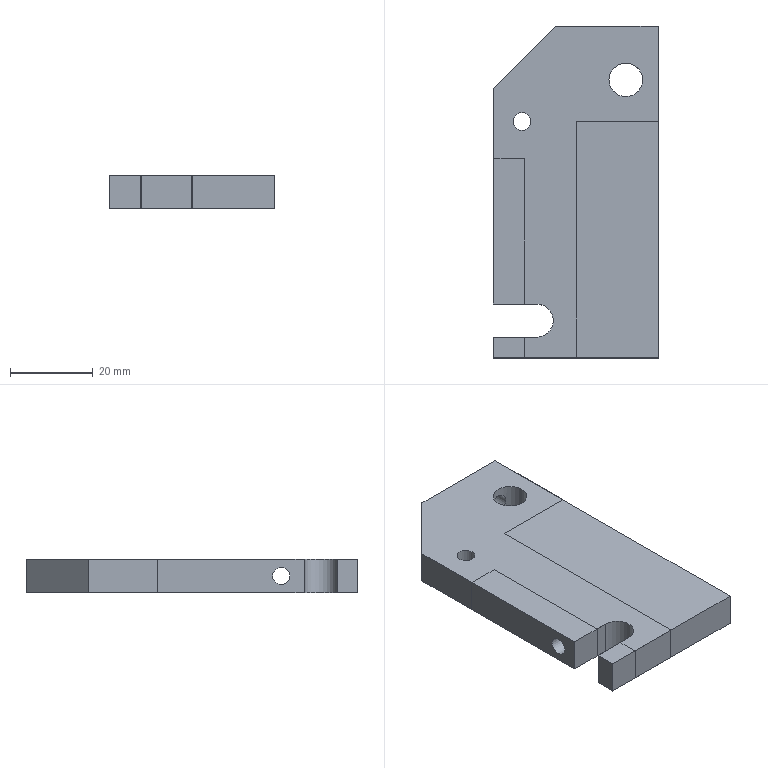NC program | NX | posted with a generic post | part box 40 x 80 x 8 mm
Whole program:
N10 G17 G21 G94 G90
(FLOOR_FACING , TOOL : D10-30-D10-75-3T-ROUGH)
N12 T01 M6
N14 G54
N16 G17 G0 G90 X-2.6 Y8.1 B0. C0. S3000 M3
N18 G43 Z20. H1
N20 Z2.7 B-180. C90.
N22 G94 G1 Z-0.3 F1500.
N24 Y5.1
N26 Y-13.1
N28 X-9.317
N30 Y5.1
N32 X-16.033
N34 Y-13.1
N36 X-22.75
N38 Y5.1
N40 X-29.467
N42 Y-13.1
N44 X-36.183
N46 Y5.1
N48 X-42.9
N50 Y-13.1
N52 Y-16.1
N54 Z2.7
N56 G0 Z20.
N58 X-2.6 Y8.1
N60 Z2.4
N62 G1 Z-0.6
N64 Y5.1
N66 Y-13.1
N68 X-9.317
N70 Y5.1
N72 X-16.033
N74 Y-13.1
N76 X-22.75
N78 Y5.1
N80 X-29.467
N82 Y-13.1
N84 X-36.183
N86 Y5.1
N88 X-42.9
N90 Y-13.1
N92 Y-16.1
N94 Z2.4
N96 G0 Z20.
N98 X-2.6 Y8.1
N100 Z2.1
N102 G1 Z-0.9
N104 Y5.1
N106 Y-13.1
N108 X-9.317
N110 Y5.1
N112 X-16.033
N114 Y-13.1
N116 X-22.75
N118 Y5.1
N120 X-29.467
N122 Y-13.1
N124 X-36.183
N126 Y5.1
N128 X-42.9
N130 Y-13.1
N132 Y-16.1
N134 Z2.1
N136 G0 Z20.
N138 X-2.6 Y8.1
N140 Z1.8
N142 G1 Z-1.2
N144 Y5.1
N146 Y-13.1
N148 X-9.317
N150 Y5.1
N152 X-16.033
N154 Y-13.1
N156 X-22.75
N158 Y5.1
N160 X-29.467
N162 Y-13.1
N164 X-36.183
N166 Y5.1
N168 X-42.9
N170 Y-13.1
N172 Y-16.1
N174 Z1.8
N176 G0 Z20.
N178 X-2.6 Y8.1
N180 Z1.5
N182 G1 Z-1.5
N184 Y5.1
N186 Y-13.1
N188 X-9.317
N190 Y5.1
N192 X-16.033
N194 Y-13.1
N196 X-22.75
N198 Y5.1
N200 X-29.467
N202 Y-13.1
N204 X-36.183
N206 Y5.1
N208 X-42.9
N210 Y-13.1
N212 Y-16.1
N214 Z1.5
N216 G0 Z20.
N218 X-2.6 Y8.1
N220 Z1.2
N222 G1 Z-1.8
N224 Y5.1
N226 Y-13.1
N228 X-9.317
N230 Y5.1
N232 X-16.033
N234 Y-13.1
N236 X-22.75
N238 Y5.1
N240 X-29.467
N242 Y-13.1
N244 X-36.183
N246 Y5.1
N248 X-42.9
N250 Y-13.1
N252 Y-16.1
N254 Z1.2
N256 G0 Z20.
N258 X-2.6 Y8.1
N260 Z0.9
N262 G1 Z-2.1
N264 Y5.1
N266 Y-13.1
N268 X-9.317
N270 Y5.1
N272 X-16.033
N274 Y-13.1
N276 X-22.75
N278 Y5.1
N280 X-29.467
N282 Y-13.1
N284 X-36.183
N286 Y5.1
N288 X-42.9
N290 Y-13.1
N292 Y-16.1
N294 Z0.9
N296 G0 Z20.
N298 X-2.6 Y8.1
N300 Z0.6
N302 G1 Z-2.4
N304 Y5.1
N306 Y-13.1
N308 X-9.317
N310 Y5.1
N312 X-16.033
N314 Y-13.1
N316 X-22.75
N318 Y5.1
N320 X-29.467
N322 Y-13.1
N324 X-36.183
N326 Y5.1
N328 X-42.9
N330 Y-13.1
N332 Y-16.1
N334 Z0.6
N336 G0 Z20.
N338 X-2.6 Y8.1
N340 Z0.3
N342 G1 Z-2.7
N344 Y5.1
N346 Y-13.1
N348 X-9.317
N350 Y5.1
N352 X-16.033
N354 Y-13.1
N356 X-22.75
N358 Y5.1
N360 X-29.467
N362 Y-13.1
N364 X-36.183
N366 Y5.1
N368 X-42.9
N370 Y-13.1
N372 Y-16.1
N374 Z0.3
N376 G0 Z20.
N378 X-2.6 Y8.1
N380 Z0.
N382 G1 Z-3.
N384 Y5.1
N386 Y-13.1
N388 X-9.317
N390 Y5.1
N392 X-16.033
N394 Y-13.1
N396 X-22.75
N398 Y5.1
N400 X-29.467
N402 Y-13.1
N404 X-36.183
N406 Y5.1
N408 X-42.9
N410 Y-13.1
N412 Y-16.1
N414 Z0.
N416 G0 Z20.
N418 X-2.6 Y8.1
N420 Z-0.3
N422 G1 Z-3.3
N424 Y5.1
N426 Y-13.1
N428 X-9.317
N430 Y5.1
N432 X-16.033
N434 Y-13.1
N436 X-22.75
N438 Y5.1
N440 X-29.467
N442 Y-13.1
N444 X-36.183
N446 Y5.1
N448 X-42.9
N450 Y-13.1
N452 Y-16.1
N454 Z-0.3
N456 G0 Z20.
N458 X-2.6 Y8.1
N460 Z-0.6
N462 G1 Z-3.6
N464 Y5.1
N466 Y-13.1
N468 X-9.317
N470 Y5.1
N472 X-16.033
N474 Y-13.1
N476 X-22.75
N478 Y5.1
N480 X-29.467
N482 Y-13.1
N484 X-36.183
N486 Y5.1
N488 X-42.9
N490 Y-13.1
N492 Y-16.1
N494 Z-0.6
N496 G0 Z20.
N498 X-2.6 Y8.1
N500 Z-0.9
N502 G1 Z-3.9
N504 Y5.1
N506 Y-13.1
N508 X-9.317
N510 Y5.1
N512 X-16.033
N514 Y-13.1
N516 X-22.75
N518 Y5.1
N520 X-29.467
N522 Y-13.1
N524 X-36.183
N526 Y5.1
N528 X-42.9
N530 Y-13.1
N532 Y-16.1
N534 Z-0.9
N536 G0 Z20.
N538 X-2.6 Y8.1
N540 Z-1.2
N542 G1 Z-4.2
N544 Y5.1
N546 Y-13.1
N548 X-9.317
N550 Y5.1
N552 X-16.033
N554 Y-13.1
N556 X-22.75
N558 Y5.1
N560 X-29.467
N562 Y-13.1
N564 X-36.183
N566 Y5.1
N568 X-42.9
N570 Y-13.1
N572 Y-16.1
N574 Z-1.2
N576 G0 Z20.
N578 X-2.6 Y8.1
N580 Z-1.5
N582 G1 Z-4.5
N584 Y5.1
N586 Y-13.1
N588 X-9.317
N590 Y5.1
N592 X-16.033
N594 Y-13.1
N596 X-22.75
N598 Y5.1
N600 X-29.467
N602 Y-13.1
N604 X-36.183
N606 Y5.1
N608 X-42.9
N610 Y-13.1
N612 Y-16.1
N614 Z-1.5
N616 G0 Z20.
N618 X-2.6 Y8.1
N620 Z-1.8
N622 G1 Z-4.8
N624 Y5.1
N626 Y-13.1
N628 X-9.317
N630 Y5.1
N632 X-16.033
N634 Y-13.1
N636 X-22.75
N638 Y5.1
N640 X-29.467
N642 Y-13.1
N644 X-36.183
N646 Y5.1
N648 X-42.9
N650 Y-13.1
N652 Y-16.1
N654 Z-1.8
N656 G0 Z20.
N658 X-2.6 Y8.1
N660 Z-2.1
N662 G1 Z-5.1
N664 Y5.1
N666 Y-13.1
N668 X-9.317
N670 Y5.1
N672 X-16.033
N674 Y-13.1
N676 X-22.75
N678 Y5.1
N680 X-29.467
N682 Y-13.1
N684 X-36.183
N686 Y5.1
N688 X-42.9
N690 Y-13.1
N692 Y-16.1
N694 Z-2.1
N696 G0 Z20.
N698 X-2.6 Y8.1
N700 Z-2.4
N702 G1 Z-5.4
N704 Y5.1
N706 Y-13.1
N708 X-9.317
N710 Y5.1
N712 X-16.033
N714 Y-13.1
N716 X-22.75
N718 Y5.1
N720 X-29.467
N722 Y-13.1
N724 X-36.183
N726 Y5.1
N728 X-42.9
N730 Y-13.1
N732 Y-16.1
N734 Z-2.4
N736 G0 Z20.
N738 X-2.6 Y8.1
N740 Z-2.7
N742 G1 Z-5.7
N744 Y5.1
N746 Y-13.1
N748 X-9.317
N750 Y5.1
N752 X-16.033
N754 Y-13.1
N756 X-22.75
N758 Y5.1
N760 X-29.467
N762 Y-13.1
N764 X-36.183
N766 Y5.1
N768 X-42.9
N770 Y-13.1
N772 Y-16.1
N774 Z-2.7
N776 G0 Z20.
N778 X-2.6 Y8.1
N780 Z-3.
N782 G1 Z-6.
N784 Y5.1
N786 Y-13.1
N788 X-9.317
N790 Y5.1
N792 X-16.033
N794 Y-13.1
N796 X-22.75
N798 Y5.1
N800 X-29.467
N802 Y-13.1
N804 X-36.183
N806 Y5.1
N808 X-42.9
N810 Y-13.1
N812 Y-16.1
N814 Z-3.
N816 G0 Z20.
N818 X-2.6 Y8.1
N820 Z-3.3
N822 G1 Z-6.3
N824 Y5.1
N826 Y-13.1
N828 X-9.317
N830 Y5.1
N832 X-16.033
N834 Y-13.1
N836 X-22.75
N838 Y5.1
N840 X-29.467
N842 Y-13.1
N844 X-36.183
N846 Y5.1
N848 X-42.9
N850 Y-13.1
N852 Y-16.1
N854 Z-3.3
N856 G0 Z20.
N858 X-2.6 Y8.1
N860 Z-3.6
N862 G1 Z-6.6
N864 Y5.1
N866 Y-13.1
N868 X-9.317
N870 Y5.1
N872 X-16.033
N874 Y-13.1
N876 X-22.75
N878 Y5.1
N880 X-29.467
N882 Y-13.1
N884 X-36.183
N886 Y5.1
N888 X-42.9
N890 Y-13.1
N892 Y-16.1
N894 Z-3.6
N896 G0 Z20.
N898 X-2.6 Y8.1
N900 Z-3.9
N902 G1 Z-6.9
N904 Y5.1
N906 Y-13.1
N908 X-9.317
N910 Y5.1
N912 X-16.033
N914 Y-13.1
N916 X-22.75
N918 Y5.1
N920 X-29.467
N922 Y-13.1
N924 X-36.183
N926 Y5.1
N928 X-42.9
N930 Y-13.1
N932 Y-16.1
N934 Z-3.9
N936 G0 Z20.
N938 X-2.6 Y8.1
N940 Z-4.2
N942 G1 Z-7.2
N944 Y5.1
N946 Y-13.1
N948 X-9.317
N950 Y5.1
N952 X-16.033
N954 Y-13.1
N956 X-22.75
N958 Y5.1
N960 X-29.467
N962 Y-13.1
N964 X-36.183
N966 Y5.1
N968 X-42.9
N970 Y-13.1
N972 Y-16.1
N974 Z-4.2
N976 G0 Z20.
N978 X-2.6 Y8.1
N980 Z-4.5
N982 G1 Z-7.5
N984 Y5.1
N986 Y-13.1
N988 X-9.317
N990 Y5.1
N992 X-16.033
N994 Y-13.1
N996 X-22.75
N998 Y5.1
N1000 X-29.467
N1002 Y-13.1
N1004 X-36.183
N1006 Y5.1
N1008 X-42.9
N1010 Y-13.1
N1012 Y-16.1
N1014 Z-4.5
N1016 G0 Z20.
N1018 M5
(FLOOR_FACING_COPY , TOOL : D6-18-D6-50-3T-FINISH)
N1020 T06 M6
N1022 G54
N1024 G17 G0 G90 X-1.7 Y6. B0. C0. S3000 M3
N1026 G43 Z20. H6
N1028 Z-4.6 B-180. C90.
N1030 G94 G1 Z-7.6 F600.
N1032 Y3.
N1034 Y-11.
N1036 X-6.025
N1038 Y3.
N1040 X-10.35
N1042 Y-11.
N1044 X-14.675
N1046 Y3.
N1048 X-19.
N1050 Y-11.
N1052 X-23.325
N1054 Y3.
N1056 X-27.65
N1058 Y-11.
N1060 X-31.975
N1062 Y3.
N1064 X-36.3
N1066 Y-11.
N1068 X-40.625
N1070 Y3.
N1072 X-44.95
N1074 Y-11.
N1076 Y-14.05
N1078 Z-4.6
N1080 G0 Z20.
(FLOOR_FACING_COPY_COPY , TOOL : D6-18-D6-50-3T-FINISH)
N1082 X-45. Y6.
N1084 Z-4.6
N1086 G1 Z-7.6
N1088 Y-1.5
N1090 Y-6.5
N1092 Y-14.
N1094 Z-4.6
N1096 G0 Z20.
N1098 M5
(PLANAR_MILL_6_COPY , TOOL : 倒角D4-90度)
N1100 T05 M6
N1102 G54
N1104 G17 G0 G90 X-11.413 Y3.992 B0. C0. S3000 M3
N1106 G43 Z20. H5
N1108 Z-7.1 B-180. C90.
N1110 G94 G1 Z-9.1 F800.
N1112 G41 X-11.5 Y3.5 D5
N1114 Y0.
N1116 Y-8.
N1118 Y-11.5
N1120 G40
N1122 X-11.413 Y-11.992
N1124 Z-7.1
N1126 G0 Z20.
N1128 X-6.587
N1130 Z-7.1
N1132 G1 Z-9.1
N1134 G41 X-6.5 Y-11.5
N1136 Y-8.
N1138 Y0.
N1140 Y3.5
N1142 G40
N1144 X-6.587 Y3.992
N1146 Z-7.1
N1148 G0 Z20.
N1150 X1.587
N1152 Z-7.1
N1154 G1 Z-9.1
N1156 G41 X1.5 Y3.5
N1158 Y0.
N1160 Y-8.
N1162 Y-11.5
N1164 G40
N1166 X1.587 Y-11.992
N1168 Z-7.1
N1170 G0 Z20.
(PLANAR_MILL_6 , TOOL : 倒角D4-90度)
N1172 X-46.413 Y3.992
N1174 Z0.5
N1176 G1 Z-1.5
N1178 G41 X-46.5 Y3.5
N1180 Y0.
N1182 Y-8.
N1184 Y-11.5
N1186 G40
N1188 X-46.413 Y-11.992
N1190 Z0.5
N1192 G0 Z20.
N1194 M5
N1196 M2